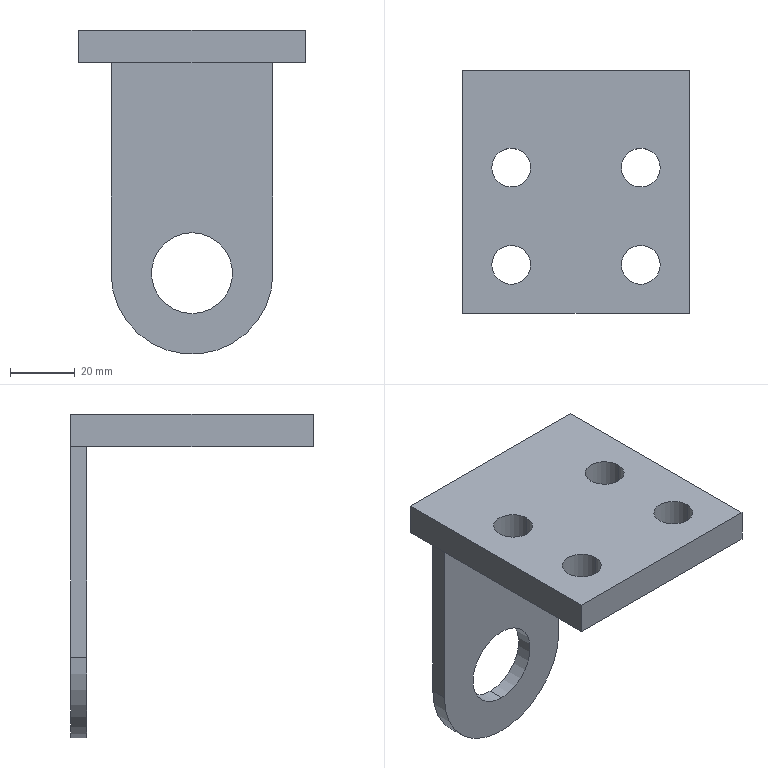Part | SolidWorks | features ICE 2, Extrusion 1 | 1 solid | 20 faces | box 70 x 75 x 100 mm | volume 66680 mm3 | cylinder 11 | plane 9 | commonest cylinder face diameters 12 x8 25 x2 50 x1
STEP:
#1=CARTESIAN_POINT('',(20.,55.,-52.5));
#2=VERTEX_POINT('',#1);
#3=CARTESIAN_POINT('',(20.,55.,-77.5));
#4=VERTEX_POINT('',#3);
#5=CARTESIAN_POINT('',(20.,55.,-65.));
#6=DIRECTION('',(0.,-1.,0.));
#7=DIRECTION('',(0.,0.,-1.));
#8=AXIS2_PLACEMENT_3D('',#5,#6,#7);
#9=CIRCLE('',#8,12.5);
#10=EDGE_CURVE('',#2,#4,#9,.T.);
#11=ORIENTED_EDGE('',*,*,#10,.T.);
#12=CARTESIAN_POINT('',(20.,60.,-77.5));
#13=VERTEX_POINT('',#12);
#14=CARTESIAN_POINT('',(20.,50.,-77.5));
#15=DIRECTION('',(0.,1.,0.));
#16=VECTOR('',#15,1000.);
#17=LINE('',#14,#16);
#18=EDGE_CURVE('',#4,#13,#17,.T.);
#19=ORIENTED_EDGE('',*,*,#18,.T.);
#20=CARTESIAN_POINT('',(20.,60.,-52.5));
#21=VERTEX_POINT('',#20);
#22=CARTESIAN_POINT('',(20.,60.,-65.));
#23=DIRECTION('',(0.,1.,0.));
#24=DIRECTION('',(0.,0.,1.));
#25=AXIS2_PLACEMENT_3D('',#22,#23,#24);
#26=CIRCLE('',#25,12.5);
#27=EDGE_CURVE('',#13,#21,#26,.T.);
#28=ORIENTED_EDGE('',*,*,#27,.T.);
#29=CARTESIAN_POINT('',(20.,50.,-52.5));
#30=DIRECTION('',(0.,1.,0.));
#31=VECTOR('',#30,1000.);
#32=LINE('',#29,#31);
#33=EDGE_CURVE('',#2,#21,#32,.T.);
#34=ORIENTED_EDGE('',*,*,#33,.F.);
#35=EDGE_LOOP('',(#11,#19,#28,#34));
#36=FACE_OUTER_BOUND('',#35,.T.);
#37=CARTESIAN_POINT('',(20.,50.,-65.));
#38=DIRECTION('',(0.,1.,0.));
#39=DIRECTION('',(0.,0.,1.));
#40=AXIS2_PLACEMENT_3D('',#37,#38,#39);
#41=CYLINDRICAL_SURFACE('',#40,12.5);
#42=ADVANCED_FACE('',(#36),#41,.F.);
#43=CARTESIAN_POINT('',(34.,0.,10.));
#44=VERTEX_POINT('',#43);
#45=CARTESIAN_POINT('',(46.,0.,10.));
#46=VERTEX_POINT('',#45);
#47=CARTESIAN_POINT('',(40.,0.,10.));
#48=DIRECTION('',(0.,0.,1.));
#49=DIRECTION('',(1.,0.,0.));
#50=AXIS2_PLACEMENT_3D('',#47,#48,#49);
#51=CIRCLE('',#50,6.);
#52=EDGE_CURVE('',#44,#46,#51,.T.);
#53=ORIENTED_EDGE('',*,*,#52,.T.);
#54=CARTESIAN_POINT('',(46.,0.,0.));
#55=VERTEX_POINT('',#54);
#56=CARTESIAN_POINT('',(46.,0.,10.));
#57=DIRECTION('',(0.,0.,-1.));
#58=VECTOR('',#57,1000.);
#59=LINE('',#56,#58);
#60=EDGE_CURVE('',#46,#55,#59,.T.);
#61=ORIENTED_EDGE('',*,*,#60,.T.);
#62=CARTESIAN_POINT('',(34.,0.,0.));
#63=VERTEX_POINT('',#62);
#64=CARTESIAN_POINT('',(40.,0.,0.));
#65=DIRECTION('',(0.,0.,1.));
#66=DIRECTION('',(1.,0.,0.));
#67=AXIS2_PLACEMENT_3D('',#64,#65,#66);
#68=CIRCLE('',#67,6.);
#69=EDGE_CURVE('',#63,#55,#68,.T.);
#70=ORIENTED_EDGE('',*,*,#69,.F.);
#71=CARTESIAN_POINT('',(34.,0.,10.));
#72=DIRECTION('',(0.,0.,-1.));
#73=VECTOR('',#72,1000.);
#74=LINE('',#71,#73);
#75=EDGE_CURVE('',#44,#63,#74,.T.);
#76=ORIENTED_EDGE('',*,*,#75,.F.);
#77=EDGE_LOOP('',(#53,#61,#70,#76));
#78=FACE_OUTER_BOUND('',#77,.T.);
#79=CARTESIAN_POINT('',(40.,0.,10.));
#80=DIRECTION('',(0.,0.,-1.));
#81=DIRECTION('',(-1.,0.,0.));
#82=AXIS2_PLACEMENT_3D('',#79,#80,#81);
#83=CYLINDRICAL_SURFACE('',#82,6.);
#84=ADVANCED_FACE('',(#78),#83,.F.);
#85=CARTESIAN_POINT('',(34.,30.,10.));
#86=VERTEX_POINT('',#85);
#87=CARTESIAN_POINT('',(46.,30.,10.));
#88=VERTEX_POINT('',#87);
#89=CARTESIAN_POINT('',(40.,30.,10.));
#90=DIRECTION('',(0.,0.,1.));
#91=DIRECTION('',(1.,0.,0.));
#92=AXIS2_PLACEMENT_3D('',#89,#90,#91);
#93=CIRCLE('',#92,6.);
#94=EDGE_CURVE('',#86,#88,#93,.T.);
#95=ORIENTED_EDGE('',*,*,#94,.T.);
#96=CARTESIAN_POINT('',(46.,30.,0.));
#97=VERTEX_POINT('',#96);
#98=CARTESIAN_POINT('',(46.,30.,10.));
#99=DIRECTION('',(0.,0.,-1.));
#100=VECTOR('',#99,1000.);
#101=LINE('',#98,#100);
#102=EDGE_CURVE('',#88,#97,#101,.T.);
#103=ORIENTED_EDGE('',*,*,#102,.T.);
#104=CARTESIAN_POINT('',(34.,30.,0.));
#105=VERTEX_POINT('',#104);
#106=CARTESIAN_POINT('',(40.,30.,0.));
#107=DIRECTION('',(0.,0.,1.));
#108=DIRECTION('',(1.,0.,0.));
#109=AXIS2_PLACEMENT_3D('',#106,#107,#108);
#110=CIRCLE('',#109,6.);
#111=EDGE_CURVE('',#105,#97,#110,.T.);
#112=ORIENTED_EDGE('',*,*,#111,.F.);
#113=CARTESIAN_POINT('',(34.,30.,10.));
#114=DIRECTION('',(0.,0.,-1.));
#115=VECTOR('',#114,1000.);
#116=LINE('',#113,#115);
#117=EDGE_CURVE('',#86,#105,#116,.T.);
#118=ORIENTED_EDGE('',*,*,#117,.F.);
#119=EDGE_LOOP('',(#95,#103,#112,#118));
#120=FACE_OUTER_BOUND('',#119,.T.);
#121=CARTESIAN_POINT('',(40.,30.,10.));
#122=DIRECTION('',(0.,0.,-1.));
#123=DIRECTION('',(-1.,0.,0.));
#124=AXIS2_PLACEMENT_3D('',#121,#122,#123);
#125=CYLINDRICAL_SURFACE('',#124,6.);
#126=ADVANCED_FACE('',(#120),#125,.F.);
#127=CARTESIAN_POINT('',(-6.,30.,10.));
#128=VERTEX_POINT('',#127);
#129=CARTESIAN_POINT('',(6.,30.,10.));
#130=VERTEX_POINT('',#129);
#131=CARTESIAN_POINT('',(0.,30.,10.));
#132=DIRECTION('',(0.,0.,1.));
#133=DIRECTION('',(1.,0.,0.));
#134=AXIS2_PLACEMENT_3D('',#131,#132,#133);
#135=CIRCLE('',#134,6.);
#136=EDGE_CURVE('',#128,#130,#135,.T.);
#137=ORIENTED_EDGE('',*,*,#136,.T.);
#138=CARTESIAN_POINT('',(6.,30.,0.));
#139=VERTEX_POINT('',#138);
#140=CARTESIAN_POINT('',(6.,30.,10.));
#141=DIRECTION('',(0.,0.,-1.));
#142=VECTOR('',#141,1000.);
#143=LINE('',#140,#142);
#144=EDGE_CURVE('',#130,#139,#143,.T.);
#145=ORIENTED_EDGE('',*,*,#144,.T.);
#146=CARTESIAN_POINT('',(-6.,30.,0.));
#147=VERTEX_POINT('',#146);
#148=CARTESIAN_POINT('',(0.,30.,0.));
#149=DIRECTION('',(0.,0.,1.));
#150=DIRECTION('',(1.,0.,0.));
#151=AXIS2_PLACEMENT_3D('',#148,#149,#150);
#152=CIRCLE('',#151,6.);
#153=EDGE_CURVE('',#147,#139,#152,.T.);
#154=ORIENTED_EDGE('',*,*,#153,.F.);
#155=CARTESIAN_POINT('',(-6.,30.,10.));
#156=DIRECTION('',(0.,0.,-1.));
#157=VECTOR('',#156,1000.);
#158=LINE('',#155,#157);
#159=EDGE_CURVE('',#128,#147,#158,.T.);
#160=ORIENTED_EDGE('',*,*,#159,.F.);
#161=EDGE_LOOP('',(#137,#145,#154,#160));
#162=FACE_OUTER_BOUND('',#161,.T.);
#163=CARTESIAN_POINT('',(0.,30.,10.));
#164=DIRECTION('',(0.,0.,-1.));
#165=DIRECTION('',(-1.,0.,0.));
#166=AXIS2_PLACEMENT_3D('',#163,#164,#165);
#167=CYLINDRICAL_SURFACE('',#166,6.);
#168=ADVANCED_FACE('',(#162),#167,.F.);
#169=CARTESIAN_POINT('',(-6.,0.,10.));
#170=VERTEX_POINT('',#169);
#171=CARTESIAN_POINT('',(6.,0.,10.));
#172=VERTEX_POINT('',#171);
#173=CARTESIAN_POINT('',(0.,0.,10.));
#174=DIRECTION('',(0.,0.,1.));
#175=DIRECTION('',(1.,0.,0.));
#176=AXIS2_PLACEMENT_3D('',#173,#174,#175);
#177=CIRCLE('',#176,6.);
#178=EDGE_CURVE('',#170,#172,#177,.T.);
#179=ORIENTED_EDGE('',*,*,#178,.T.);
#180=CARTESIAN_POINT('',(6.,0.,0.));
#181=VERTEX_POINT('',#180);
#182=CARTESIAN_POINT('',(6.,0.,10.));
#183=DIRECTION('',(0.,0.,-1.));
#184=VECTOR('',#183,1000.);
#185=LINE('',#182,#184);
#186=EDGE_CURVE('',#172,#181,#185,.T.);
#187=ORIENTED_EDGE('',*,*,#186,.T.);
#188=CARTESIAN_POINT('',(-6.,0.,0.));
#189=VERTEX_POINT('',#188);
#190=CARTESIAN_POINT('',(0.,0.,0.));
#191=DIRECTION('',(0.,0.,1.));
#192=DIRECTION('',(1.,0.,0.));
#193=AXIS2_PLACEMENT_3D('',#190,#191,#192);
#194=CIRCLE('',#193,6.);
#195=EDGE_CURVE('',#189,#181,#194,.T.);
#196=ORIENTED_EDGE('',*,*,#195,.F.);
#197=CARTESIAN_POINT('',(-6.,0.,10.));
#198=DIRECTION('',(0.,0.,-1.));
#199=VECTOR('',#198,1000.);
#200=LINE('',#197,#199);
#201=EDGE_CURVE('',#170,#189,#200,.T.);
#202=ORIENTED_EDGE('',*,*,#201,.F.);
#203=EDGE_LOOP('',(#179,#187,#196,#202));
#204=FACE_OUTER_BOUND('',#203,.T.);
#205=CARTESIAN_POINT('',(0.,0.,10.));
#206=DIRECTION('',(0.,0.,-1.));
#207=DIRECTION('',(-1.,0.,0.));
#208=AXIS2_PLACEMENT_3D('',#205,#206,#207);
#209=CYLINDRICAL_SURFACE('',#208,6.);
#210=ADVANCED_FACE('',(#204),#209,.F.);
#211=ORIENTED_EDGE('',*,*,#94,.F.);
#212=CARTESIAN_POINT('',(40.,30.,10.));
#213=DIRECTION('',(0.,0.,1.));
#214=DIRECTION('',(1.,0.,0.));
#215=AXIS2_PLACEMENT_3D('',#212,#213,#214);
#216=CIRCLE('',#215,6.);
#217=EDGE_CURVE('',#88,#86,#216,.T.);
#218=ORIENTED_EDGE('',*,*,#217,.F.);
#219=EDGE_LOOP('',(#211,#218));
#220=FACE_BOUND('',#219,.T.);
#221=ORIENTED_EDGE('',*,*,#178,.F.);
#222=CARTESIAN_POINT('',(0.,0.,10.));
#223=DIRECTION('',(0.,0.,1.));
#224=DIRECTION('',(1.,0.,0.));
#225=AXIS2_PLACEMENT_3D('',#222,#223,#224);
#226=CIRCLE('',#225,6.);
#227=EDGE_CURVE('',#172,#170,#226,.T.);
#228=ORIENTED_EDGE('',*,*,#227,.F.);
#229=EDGE_LOOP('',(#221,#228));
#230=FACE_BOUND('',#229,.T.);
#231=CARTESIAN_POINT('',(-15.,60.,10.));
#232=VERTEX_POINT('',#231);
#233=CARTESIAN_POINT('',(-15.,-15.,10.));
#234=VERTEX_POINT('',#233);
#235=CARTESIAN_POINT('',(-15.,55.,10.));
#236=DIRECTION('',(0.,-1.,0.));
#237=VECTOR('',#236,1000.);
#238=LINE('',#235,#237);
#239=EDGE_CURVE('',#232,#234,#238,.T.);
#240=ORIENTED_EDGE('',*,*,#239,.T.);
#241=CARTESIAN_POINT('',(55.,-15.,10.));
#242=VERTEX_POINT('',#241);
#243=CARTESIAN_POINT('',(-15.,-15.,10.));
#244=DIRECTION('',(1.,0.,0.));
#245=VECTOR('',#244,1000.);
#246=LINE('',#243,#245);
#247=EDGE_CURVE('',#234,#242,#246,.T.);
#248=ORIENTED_EDGE('',*,*,#247,.T.);
#249=CARTESIAN_POINT('',(55.,60.,10.));
#250=VERTEX_POINT('',#249);
#251=CARTESIAN_POINT('',(55.,55.,10.));
#252=DIRECTION('',(0.,1.,0.));
#253=VECTOR('',#252,1000.);
#254=LINE('',#251,#253);
#255=EDGE_CURVE('',#242,#250,#254,.T.);
#256=ORIENTED_EDGE('',*,*,#255,.T.);
#257=CARTESIAN_POINT('',(-15.,60.,10.));
#258=DIRECTION('',(-1.,0.,0.));
#259=VECTOR('',#258,1000.);
#260=LINE('',#257,#259);
#261=EDGE_CURVE('',#250,#232,#260,.T.);
#262=ORIENTED_EDGE('',*,*,#261,.T.);
#263=EDGE_LOOP('',(#240,#248,#256,#262));
#264=FACE_OUTER_BOUND('',#263,.T.);
#265=ORIENTED_EDGE('',*,*,#136,.F.);
#266=CARTESIAN_POINT('',(0.,30.,10.));
#267=DIRECTION('',(0.,0.,1.));
#268=DIRECTION('',(1.,0.,0.));
#269=AXIS2_PLACEMENT_3D('',#266,#267,#268);
#270=CIRCLE('',#269,6.);
#271=EDGE_CURVE('',#130,#128,#270,.T.);
#272=ORIENTED_EDGE('',*,*,#271,.F.);
#273=EDGE_LOOP('',(#265,#272));
#274=FACE_BOUND('',#273,.T.);
#275=ORIENTED_EDGE('',*,*,#52,.F.);
#276=CARTESIAN_POINT('',(40.,0.,10.));
#277=DIRECTION('',(0.,0.,1.));
#278=DIRECTION('',(1.,0.,0.));
#279=AXIS2_PLACEMENT_3D('',#276,#277,#278);
#280=CIRCLE('',#279,6.);
#281=EDGE_CURVE('',#46,#44,#280,.T.);
#282=ORIENTED_EDGE('',*,*,#281,.F.);
#283=EDGE_LOOP('',(#275,#282));
#284=FACE_BOUND('',#283,.T.);
#285=CARTESIAN_POINT('',(0.,0.,10.));
#286=DIRECTION('',(0.,0.,1.));
#287=DIRECTION('',(1.,0.,0.));
#288=AXIS2_PLACEMENT_3D('',#285,#286,#287);
#289=PLANE('',#288);
#290=ADVANCED_FACE('',(#220,#230,#264,#274,#284),#289,.T.);
#291=CARTESIAN_POINT('',(-5.,55.,0.));
#292=VERTEX_POINT('',#291);
#293=CARTESIAN_POINT('',(-5.,60.,0.));
#294=VERTEX_POINT('',#293);
#295=CARTESIAN_POINT('',(-5.,50.,0.));
#296=DIRECTION('',(0.,1.,0.));
#297=VECTOR('',#296,1000.);
#298=LINE('',#295,#297);
#299=EDGE_CURVE('',#292,#294,#298,.T.);
#300=ORIENTED_EDGE('',*,*,#299,.F.);
#301=CARTESIAN_POINT('',(45.,55.,0.));
#302=VERTEX_POINT('',#301);
#303=CARTESIAN_POINT('',(-15.,55.,0.));
#304=DIRECTION('',(-1.,0.,0.));
#305=VECTOR('',#304,1000.);
#306=LINE('',#303,#305);
#307=EDGE_CURVE('',#302,#292,#306,.T.);
#308=ORIENTED_EDGE('',*,*,#307,.F.);
#309=CARTESIAN_POINT('',(45.,60.,0.));
#310=VERTEX_POINT('',#309);
#311=CARTESIAN_POINT('',(45.,50.,0.));
#312=DIRECTION('',(0.,1.,0.));
#313=VECTOR('',#312,1000.);
#314=LINE('',#311,#313);
#315=EDGE_CURVE('',#302,#310,#314,.T.);
#316=ORIENTED_EDGE('',*,*,#315,.T.);
#317=CARTESIAN_POINT('',(55.,60.,0.));
#318=VERTEX_POINT('',#317);
#319=CARTESIAN_POINT('',(45.,60.,0.));
#320=DIRECTION('',(1.,0.,0.));
#321=VECTOR('',#320,1000.);
#322=LINE('',#319,#321);
#323=EDGE_CURVE('',#310,#318,#322,.T.);
#324=ORIENTED_EDGE('',*,*,#323,.T.);
#325=CARTESIAN_POINT('',(55.,-15.,0.));
#326=VERTEX_POINT('',#325);
#327=CARTESIAN_POINT('',(55.,55.,0.));
#328=DIRECTION('',(0.,1.,0.));
#329=VECTOR('',#328,1000.);
#330=LINE('',#327,#329);
#331=EDGE_CURVE('',#326,#318,#330,.T.);
#332=ORIENTED_EDGE('',*,*,#331,.F.);
#333=CARTESIAN_POINT('',(-15.,-15.,0.));
#334=VERTEX_POINT('',#333);
#335=CARTESIAN_POINT('',(-15.,-15.,0.));
#336=DIRECTION('',(1.,0.,0.));
#337=VECTOR('',#336,1000.);
#338=LINE('',#335,#337);
#339=EDGE_CURVE('',#334,#326,#338,.T.);
#340=ORIENTED_EDGE('',*,*,#339,.F.);
#341=CARTESIAN_POINT('',(-15.,60.,0.));
#342=VERTEX_POINT('',#341);
#343=CARTESIAN_POINT('',(-15.,55.,0.));
#344=DIRECTION('',(0.,-1.,0.));
#345=VECTOR('',#344,1000.);
#346=LINE('',#343,#345);
#347=EDGE_CURVE('',#342,#334,#346,.T.);
#348=ORIENTED_EDGE('',*,*,#347,.F.);
#349=CARTESIAN_POINT('',(-5.,60.,0.));
#350=DIRECTION('',(1.,0.,0.));
#351=VECTOR('',#350,1000.);
#352=LINE('',#349,#351);
#353=EDGE_CURVE('',#342,#294,#352,.T.);
#354=ORIENTED_EDGE('',*,*,#353,.T.);
#355=EDGE_LOOP('',(#300,#308,#316,#324,#332,#340,#348,#354));
#356=FACE_OUTER_BOUND('',#355,.T.);
#357=ORIENTED_EDGE('',*,*,#111,.T.);
#358=CARTESIAN_POINT('',(40.,30.,0.));
#359=DIRECTION('',(0.,0.,1.));
#360=DIRECTION('',(1.,0.,0.));
#361=AXIS2_PLACEMENT_3D('',#358,#359,#360);
#362=CIRCLE('',#361,6.);
#363=EDGE_CURVE('',#97,#105,#362,.T.);
#364=ORIENTED_EDGE('',*,*,#363,.T.);
#365=EDGE_LOOP('',(#357,#364));
#366=FACE_BOUND('',#365,.T.);
#367=ORIENTED_EDGE('',*,*,#195,.T.);
#368=CARTESIAN_POINT('',(0.,0.,0.));
#369=DIRECTION('',(0.,0.,1.));
#370=DIRECTION('',(1.,0.,0.));
#371=AXIS2_PLACEMENT_3D('',#368,#369,#370);
#372=CIRCLE('',#371,6.);
#373=EDGE_CURVE('',#181,#189,#372,.T.);
#374=ORIENTED_EDGE('',*,*,#373,.T.);
#375=EDGE_LOOP('',(#367,#374));
#376=FACE_BOUND('',#375,.T.);
#377=ORIENTED_EDGE('',*,*,#153,.T.);
#378=CARTESIAN_POINT('',(0.,30.,0.));
#379=DIRECTION('',(0.,0.,1.));
#380=DIRECTION('',(1.,0.,0.));
#381=AXIS2_PLACEMENT_3D('',#378,#379,#380);
#382=CIRCLE('',#381,6.);
#383=EDGE_CURVE('',#139,#147,#382,.T.);
#384=ORIENTED_EDGE('',*,*,#383,.T.);
#385=EDGE_LOOP('',(#377,#384));
#386=FACE_BOUND('',#385,.T.);
#387=ORIENTED_EDGE('',*,*,#69,.T.);
#388=CARTESIAN_POINT('',(40.,0.,0.));
#389=DIRECTION('',(0.,0.,1.));
#390=DIRECTION('',(1.,0.,0.));
#391=AXIS2_PLACEMENT_3D('',#388,#389,#390);
#392=CIRCLE('',#391,6.);
#393=EDGE_CURVE('',#55,#63,#392,.T.);
#394=ORIENTED_EDGE('',*,*,#393,.T.);
#395=EDGE_LOOP('',(#387,#394));
#396=FACE_BOUND('',#395,.T.);
#397=CARTESIAN_POINT('',(0.,0.,0.));
#398=DIRECTION('',(0.,0.,1.));
#399=DIRECTION('',(1.,0.,0.));
#400=AXIS2_PLACEMENT_3D('',#397,#398,#399);
#401=PLANE('',#400);
#402=ADVANCED_FACE('',(#356,#366,#376,#386,#396),#401,.F.);
#403=CARTESIAN_POINT('',(-15.,60.,-90.));
#404=DIRECTION('',(0.,0.,1.));
#405=VECTOR('',#404,1000.);
#406=LINE('',#403,#405);
#407=EDGE_CURVE('',#342,#232,#406,.T.);
#408=ORIENTED_EDGE('',*,*,#407,.F.);
#409=ORIENTED_EDGE('',*,*,#347,.T.);
#410=CARTESIAN_POINT('',(-15.,-15.,10.));
#411=DIRECTION('',(0.,0.,-1.));
#412=VECTOR('',#411,1000.);
#413=LINE('',#410,#412);
#414=EDGE_CURVE('',#234,#334,#413,.T.);
#415=ORIENTED_EDGE('',*,*,#414,.F.);
#416=ORIENTED_EDGE('',*,*,#239,.F.);
#417=EDGE_LOOP('',(#408,#409,#415,#416));
#418=FACE_OUTER_BOUND('',#417,.T.);
#419=CARTESIAN_POINT('',(-15.,55.,10.));
#420=DIRECTION('',(1.,0.,0.));
#421=DIRECTION('',(0.,1.,0.));
#422=AXIS2_PLACEMENT_3D('',#419,#420,#421);
#423=PLANE('',#422);
#424=ADVANCED_FACE('',(#418),#423,.F.);
#425=ORIENTED_EDGE('',*,*,#339,.T.);
#426=CARTESIAN_POINT('',(55.,-15.,10.));
#427=DIRECTION('',(0.,0.,-1.));
#428=VECTOR('',#427,1000.);
#429=LINE('',#426,#428);
#430=EDGE_CURVE('',#242,#326,#429,.T.);
#431=ORIENTED_EDGE('',*,*,#430,.F.);
#432=ORIENTED_EDGE('',*,*,#247,.F.);
#433=ORIENTED_EDGE('',*,*,#414,.T.);
#434=EDGE_LOOP('',(#425,#431,#432,#433));
#435=FACE_OUTER_BOUND('',#434,.T.);
#436=CARTESIAN_POINT('',(-15.,-15.,10.));
#437=DIRECTION('',(0.,1.,0.));
#438=DIRECTION('',(0.,0.,1.));
#439=AXIS2_PLACEMENT_3D('',#436,#437,#438);
#440=PLANE('',#439);
#441=ADVANCED_FACE('',(#435),#440,.F.);
#442=ORIENTED_EDGE('',*,*,#331,.T.);
#443=CARTESIAN_POINT('',(55.,60.,-90.));
#444=DIRECTION('',(0.,0.,1.));
#445=VECTOR('',#444,1000.);
#446=LINE('',#443,#445);
#447=EDGE_CURVE('',#318,#250,#446,.T.);
#448=ORIENTED_EDGE('',*,*,#447,.T.);
#449=ORIENTED_EDGE('',*,*,#255,.F.);
#450=ORIENTED_EDGE('',*,*,#430,.T.);
#451=EDGE_LOOP('',(#442,#448,#449,#450));
#452=FACE_OUTER_BOUND('',#451,.T.);
#453=CARTESIAN_POINT('',(55.,55.,10.));
#454=DIRECTION('',(-1.,0.,0.));
#455=DIRECTION('',(0.,-1.,0.));
#456=AXIS2_PLACEMENT_3D('',#453,#454,#455);
#457=PLANE('',#456);
#458=ADVANCED_FACE('',(#452),#457,.F.);
#459=ORIENTED_EDGE('',*,*,#186,.F.);
#460=ORIENTED_EDGE('',*,*,#227,.T.);
#461=ORIENTED_EDGE('',*,*,#201,.T.);
#462=ORIENTED_EDGE('',*,*,#373,.F.);
#463=EDGE_LOOP('',(#459,#460,#461,#462));
#464=FACE_OUTER_BOUND('',#463,.T.);
#465=CARTESIAN_POINT('',(0.,0.,10.));
#466=DIRECTION('',(0.,0.,-1.));
#467=DIRECTION('',(-1.,0.,0.));
#468=AXIS2_PLACEMENT_3D('',#465,#466,#467);
#469=CYLINDRICAL_SURFACE('',#468,6.);
#470=ADVANCED_FACE('',(#464),#469,.F.);
#471=ORIENTED_EDGE('',*,*,#144,.F.);
#472=ORIENTED_EDGE('',*,*,#271,.T.);
#473=ORIENTED_EDGE('',*,*,#159,.T.);
#474=ORIENTED_EDGE('',*,*,#383,.F.);
#475=EDGE_LOOP('',(#471,#472,#473,#474));
#476=FACE_OUTER_BOUND('',#475,.T.);
#477=CARTESIAN_POINT('',(0.,30.,10.));
#478=DIRECTION('',(0.,0.,-1.));
#479=DIRECTION('',(-1.,0.,0.));
#480=AXIS2_PLACEMENT_3D('',#477,#478,#479);
#481=CYLINDRICAL_SURFACE('',#480,6.);
#482=ADVANCED_FACE('',(#476),#481,.F.);
#483=ORIENTED_EDGE('',*,*,#102,.F.);
#484=ORIENTED_EDGE('',*,*,#217,.T.);
#485=ORIENTED_EDGE('',*,*,#117,.T.);
#486=ORIENTED_EDGE('',*,*,#363,.F.);
#487=EDGE_LOOP('',(#483,#484,#485,#486));
#488=FACE_OUTER_BOUND('',#487,.T.);
#489=CARTESIAN_POINT('',(40.,30.,10.));
#490=DIRECTION('',(0.,0.,-1.));
#491=DIRECTION('',(-1.,0.,0.));
#492=AXIS2_PLACEMENT_3D('',#489,#490,#491);
#493=CYLINDRICAL_SURFACE('',#492,6.);
#494=ADVANCED_FACE('',(#488),#493,.F.);
#495=ORIENTED_EDGE('',*,*,#60,.F.);
#496=ORIENTED_EDGE('',*,*,#281,.T.);
#497=ORIENTED_EDGE('',*,*,#75,.T.);
#498=ORIENTED_EDGE('',*,*,#393,.F.);
#499=EDGE_LOOP('',(#495,#496,#497,#498));
#500=FACE_OUTER_BOUND('',#499,.T.);
#501=CARTESIAN_POINT('',(40.,0.,10.));
#502=DIRECTION('',(0.,0.,-1.));
#503=DIRECTION('',(-1.,0.,0.));
#504=AXIS2_PLACEMENT_3D('',#501,#502,#503);
#505=CYLINDRICAL_SURFACE('',#504,6.);
#506=ADVANCED_FACE('',(#500),#505,.F.);
#507=ORIENTED_EDGE('',*,*,#353,.F.);
#508=ORIENTED_EDGE('',*,*,#407,.T.);
#509=ORIENTED_EDGE('',*,*,#261,.F.);
#510=ORIENTED_EDGE('',*,*,#447,.F.);
#511=ORIENTED_EDGE('',*,*,#323,.F.);
#512=CARTESIAN_POINT('',(45.,60.,-65.));
#513=VERTEX_POINT('',#512);
#514=CARTESIAN_POINT('',(45.,60.,-65.));
#515=DIRECTION('',(0.,0.,1.));
#516=VECTOR('',#515,1000.);
#517=LINE('',#514,#516);
#518=EDGE_CURVE('',#513,#310,#517,.T.);
#519=ORIENTED_EDGE('',*,*,#518,.F.);
#520=CARTESIAN_POINT('',(-5.,60.,-65.));
#521=VERTEX_POINT('',#520);
#522=CARTESIAN_POINT('',(20.,60.,-65.));
#523=DIRECTION('',(0.,-1.,0.));
#524=DIRECTION('',(0.,0.,1.));
#525=AXIS2_PLACEMENT_3D('',#522,#523,#524);
#526=CIRCLE('',#525,25.);
#527=EDGE_CURVE('',#521,#513,#526,.T.);
#528=ORIENTED_EDGE('',*,*,#527,.F.);
#529=CARTESIAN_POINT('',(-5.,60.,-65.));
#530=DIRECTION('',(0.,0.,-1.));
#531=VECTOR('',#530,1000.);
#532=LINE('',#529,#531);
#533=EDGE_CURVE('',#294,#521,#532,.T.);
#534=ORIENTED_EDGE('',*,*,#533,.F.);
#535=EDGE_LOOP('',(#507,#508,#509,#510,#511,#519,#528,#534));
#536=FACE_OUTER_BOUND('',#535,.T.);
#537=CARTESIAN_POINT('',(20.,60.,-65.));
#538=DIRECTION('',(0.,1.,0.));
#539=DIRECTION('',(0.,0.,1.));
#540=AXIS2_PLACEMENT_3D('',#537,#538,#539);
#541=CIRCLE('',#540,12.5);
#542=EDGE_CURVE('',#21,#13,#541,.T.);
#543=ORIENTED_EDGE('',*,*,#542,.F.);
#544=ORIENTED_EDGE('',*,*,#27,.F.);
#545=EDGE_LOOP('',(#543,#544));
#546=FACE_BOUND('',#545,.T.);
#547=CARTESIAN_POINT('',(-15.,60.,-90.));
#548=DIRECTION('',(0.,1.,0.));
#549=DIRECTION('',(0.,0.,1.));
#550=AXIS2_PLACEMENT_3D('',#547,#548,#549);
#551=PLANE('',#550);
#552=ADVANCED_FACE('',(#536,#546),#551,.T.);
#553=CARTESIAN_POINT('',(-5.,55.,-65.));
#554=VERTEX_POINT('',#553);
#555=CARTESIAN_POINT('',(-5.,55.,-90.));
#556=DIRECTION('',(0.,0.,1.));
#557=VECTOR('',#556,1000.);
#558=LINE('',#555,#557);
#559=EDGE_CURVE('',#554,#292,#558,.T.);
#560=ORIENTED_EDGE('',*,*,#559,.F.);
#561=CARTESIAN_POINT('',(45.,55.,-65.));
#562=VERTEX_POINT('',#561);
#563=CARTESIAN_POINT('',(20.,55.,-65.));
#564=DIRECTION('',(0.,1.,0.));
#565=DIRECTION('',(0.,0.,-1.));
#566=AXIS2_PLACEMENT_3D('',#563,#564,#565);
#567=CIRCLE('',#566,25.);
#568=EDGE_CURVE('',#562,#554,#567,.T.);
#569=ORIENTED_EDGE('',*,*,#568,.F.);
#570=CARTESIAN_POINT('',(45.,55.,-90.));
#571=DIRECTION('',(0.,0.,-1.));
#572=VECTOR('',#571,1000.);
#573=LINE('',#570,#572);
#574=EDGE_CURVE('',#302,#562,#573,.T.);
#575=ORIENTED_EDGE('',*,*,#574,.F.);
#576=ORIENTED_EDGE('',*,*,#307,.T.);
#577=EDGE_LOOP('',(#560,#569,#575,#576));
#578=FACE_OUTER_BOUND('',#577,.T.);
#579=ORIENTED_EDGE('',*,*,#10,.F.);
#580=CARTESIAN_POINT('',(20.,55.,-65.));
#581=DIRECTION('',(0.,-1.,0.));
#582=DIRECTION('',(0.,0.,-1.));
#583=AXIS2_PLACEMENT_3D('',#580,#581,#582);
#584=CIRCLE('',#583,12.5);
#585=EDGE_CURVE('',#4,#2,#584,.T.);
#586=ORIENTED_EDGE('',*,*,#585,.F.);
#587=EDGE_LOOP('',(#579,#586));
#588=FACE_BOUND('',#587,.T.);
#589=CARTESIAN_POINT('',(-15.,55.,-90.));
#590=DIRECTION('',(0.,-1.,0.));
#591=DIRECTION('',(0.,0.,-1.));
#592=AXIS2_PLACEMENT_3D('',#589,#590,#591);
#593=PLANE('',#592);
#594=ADVANCED_FACE('',(#578,#588),#593,.T.);
#595=ORIENTED_EDGE('',*,*,#18,.F.);
#596=ORIENTED_EDGE('',*,*,#585,.T.);
#597=ORIENTED_EDGE('',*,*,#33,.T.);
#598=ORIENTED_EDGE('',*,*,#542,.T.);
#599=EDGE_LOOP('',(#595,#596,#597,#598));
#600=FACE_OUTER_BOUND('',#599,.T.);
#601=CARTESIAN_POINT('',(20.,50.,-65.));
#602=DIRECTION('',(0.,1.,0.));
#603=DIRECTION('',(0.,0.,1.));
#604=AXIS2_PLACEMENT_3D('',#601,#602,#603);
#605=CYLINDRICAL_SURFACE('',#604,12.5);
#606=ADVANCED_FACE('',(#600),#605,.F.);
#607=ORIENTED_EDGE('',*,*,#568,.T.);
#608=CARTESIAN_POINT('',(-5.,50.,-65.));
#609=DIRECTION('',(0.,1.,0.));
#610=VECTOR('',#609,1000.);
#611=LINE('',#608,#610);
#612=EDGE_CURVE('',#554,#521,#611,.T.);
#613=ORIENTED_EDGE('',*,*,#612,.T.);
#614=ORIENTED_EDGE('',*,*,#527,.T.);
#615=CARTESIAN_POINT('',(45.,50.,-65.));
#616=DIRECTION('',(0.,1.,0.));
#617=VECTOR('',#616,1000.);
#618=LINE('',#615,#617);
#619=EDGE_CURVE('',#562,#513,#618,.T.);
#620=ORIENTED_EDGE('',*,*,#619,.F.);
#621=EDGE_LOOP('',(#607,#613,#614,#620));
#622=FACE_OUTER_BOUND('',#621,.T.);
#623=CARTESIAN_POINT('',(20.,50.,-65.));
#624=DIRECTION('',(0.,1.,0.));
#625=DIRECTION('',(0.,0.,1.));
#626=AXIS2_PLACEMENT_3D('',#623,#624,#625);
#627=CYLINDRICAL_SURFACE('',#626,25.);
#628=ADVANCED_FACE('',(#622),#627,.T.);
#629=ORIENTED_EDGE('',*,*,#559,.T.);
#630=ORIENTED_EDGE('',*,*,#299,.T.);
#631=ORIENTED_EDGE('',*,*,#533,.T.);
#632=ORIENTED_EDGE('',*,*,#612,.F.);
#633=EDGE_LOOP('',(#629,#630,#631,#632));
#634=FACE_OUTER_BOUND('',#633,.T.);
#635=CARTESIAN_POINT('',(-5.,50.,-65.));
#636=DIRECTION('',(1.,0.,0.));
#637=DIRECTION('',(0.,0.,-1.));
#638=AXIS2_PLACEMENT_3D('',#635,#636,#637);
#639=PLANE('',#638);
#640=ADVANCED_FACE('',(#634),#639,.F.);
#641=ORIENTED_EDGE('',*,*,#574,.T.);
#642=ORIENTED_EDGE('',*,*,#619,.T.);
#643=ORIENTED_EDGE('',*,*,#518,.T.);
#644=ORIENTED_EDGE('',*,*,#315,.F.);
#645=EDGE_LOOP('',(#641,#642,#643,#644));
#646=FACE_OUTER_BOUND('',#645,.T.);
#647=CARTESIAN_POINT('',(45.,50.,-65.));
#648=DIRECTION('',(-1.,0.,0.));
#649=DIRECTION('',(0.,0.,1.));
#650=AXIS2_PLACEMENT_3D('',#647,#648,#649);
#651=PLANE('',#650);
#652=ADVANCED_FACE('',(#646),#651,.F.);
#653=CLOSED_SHELL('',(#42,#84,#126,#168,#210,#290,#402,#424,#441,#458,#470,#482,#494,#506,#552,#594,#606,#628,#640,#652));
#654=MANIFOLD_SOLID_BREP('',#653);
#655=CARTESIAN_POINT('',(0.,0.,0.));
#656=DIRECTION('',(0.,0.,1.));
#657=DIRECTION('',(1.,0.,0.));
#658=AXIS2_PLACEMENT_3D('',#655,#656,#657);
#659=(LENGTH_UNIT()NAMED_UNIT(*)SI_UNIT(.MILLI.,.METRE.));
#660=UNCERTAINTY_MEASURE_WITH_UNIT(LENGTH_MEASURE(0.00001),#659,'','');
#661=(NAMED_UNIT(*)PLANE_ANGLE_UNIT()SI_UNIT($,.RADIAN.));
#662=(NAMED_UNIT(*)SI_UNIT($,.STERADIAN.)SOLID_ANGLE_UNIT());
#663=(GEOMETRIC_REPRESENTATION_CONTEXT(3)GLOBAL_UNCERTAINTY_ASSIGNED_CONTEXT((#660))GLOBAL_UNIT_ASSIGNED_CONTEXT((#659,#661,#662))REPRESENTATION_CONTEXT('',''));
#664=ADVANCED_BREP_SHAPE_REPRESENTATION('',(#654,#658),#663);